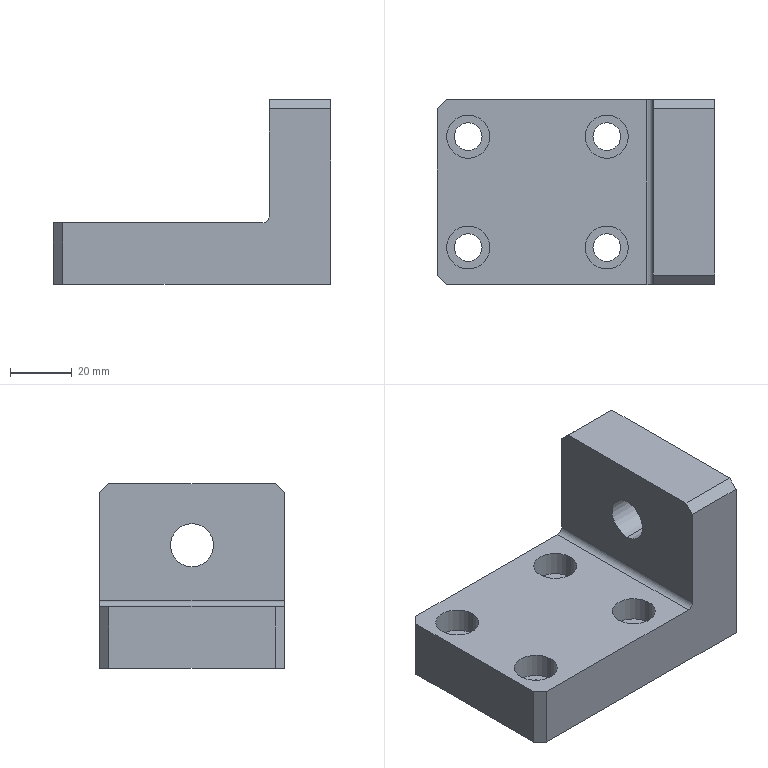Part | STEP file | Screw seat XG | 1 solid | 35 faces | box 90 x 60 x 60 mm | volume 144633 mm3 | cylinder 19 | plane 16 | commonest cylinder face diameters 14 x10 9 x8 4 x1